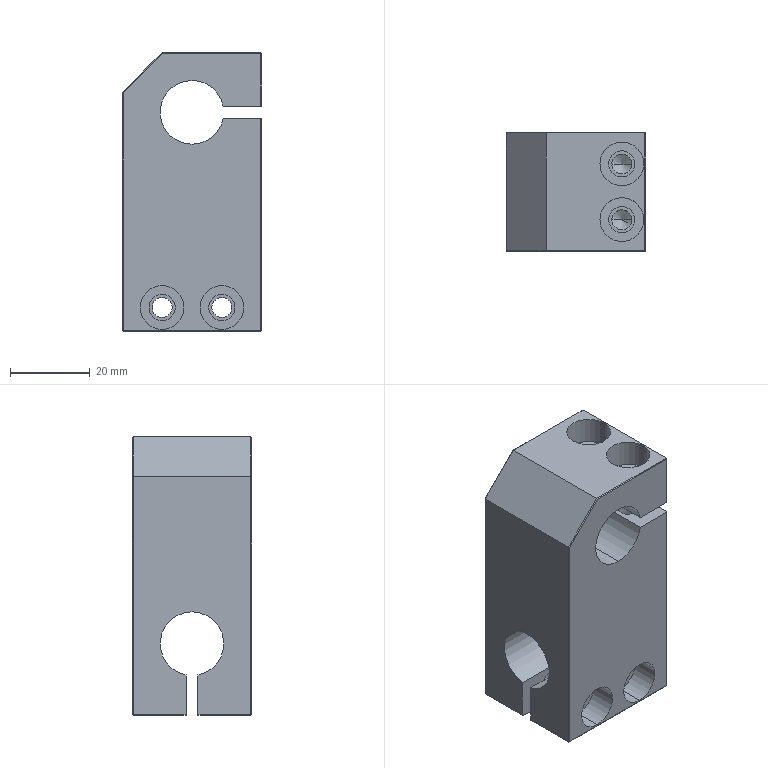Part | NX | features BREP 1 | 1 solid | 72 faces | box 35 x 30 x 70 mm | volume 52288 mm3 | plane 40 | cylinder 28 | cone 4 | commonest cylinder face diameters 5 x8 6.6 x8 11 x8 16 x4